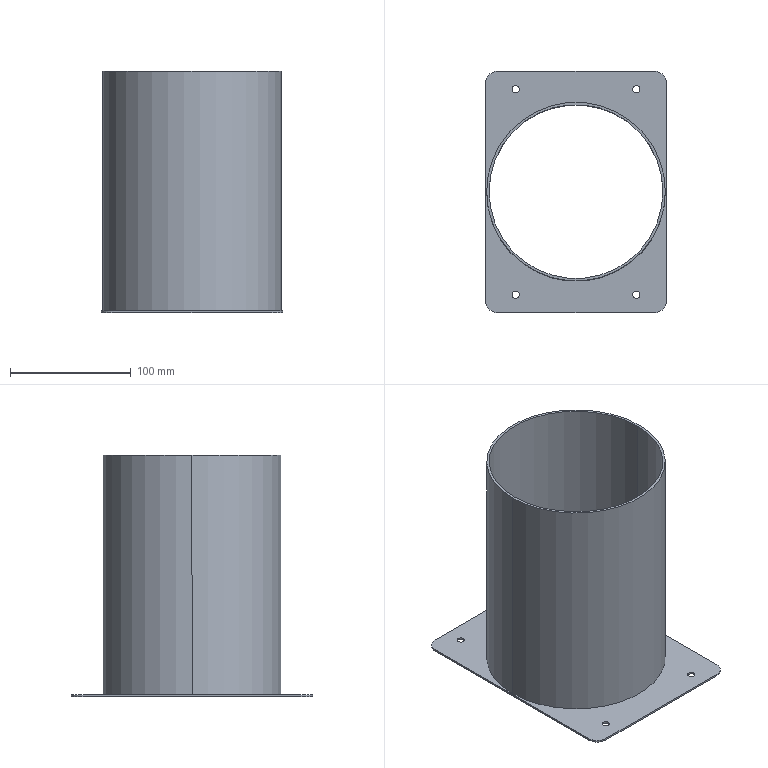Part | SolidWorks | features Extrusion 1, Fillet 1, HoleWzd 1, ICE 1 | 1 solid | 23 faces | box 150 x 200 x 200 mm | volume 202366 mm3 | cylinder 16 | plane 7 | commonest cylinder face diameters 6 x8 20 x4 144 x2 148 x2
STEP:
#1=CARTESIAN_POINT('',(-53.,-85.,0.));
#2=VERTEX_POINT('',#1);
#3=CARTESIAN_POINT('',(-47.,-85.,0.));
#4=VERTEX_POINT('',#3);
#5=CARTESIAN_POINT('',(-50.,-85.,0.));
#6=DIRECTION('',(0.,0.,1.));
#7=DIRECTION('',(1.,0.,0.));
#8=AXIS2_PLACEMENT_3D('',#5,#6,#7);
#9=CIRCLE('',#8,3.);
#10=EDGE_CURVE('',#2,#4,#9,.T.);
#11=ORIENTED_EDGE('',*,*,#10,.F.);
#12=CARTESIAN_POINT('',(-53.,-85.,1.5));
#13=VERTEX_POINT('',#12);
#14=CARTESIAN_POINT('',(-53.,-85.,1.5));
#15=DIRECTION('',(0.,0.,1.));
#16=VECTOR('',#15,1000.);
#17=LINE('',#14,#16);
#18=EDGE_CURVE('',#2,#13,#17,.T.);
#19=ORIENTED_EDGE('',*,*,#18,.T.);
#20=CARTESIAN_POINT('',(-47.,-85.,1.5));
#21=VERTEX_POINT('',#20);
#22=CARTESIAN_POINT('',(-50.,-85.,1.5));
#23=DIRECTION('',(0.,0.,1.));
#24=DIRECTION('',(1.,0.,0.));
#25=AXIS2_PLACEMENT_3D('',#22,#23,#24);
#26=CIRCLE('',#25,3.);
#27=EDGE_CURVE('',#13,#21,#26,.T.);
#28=ORIENTED_EDGE('',*,*,#27,.T.);
#29=CARTESIAN_POINT('',(-47.,-85.,1.5));
#30=DIRECTION('',(0.,0.,1.));
#31=VECTOR('',#30,1000.);
#32=LINE('',#29,#31);
#33=EDGE_CURVE('',#4,#21,#32,.T.);
#34=ORIENTED_EDGE('',*,*,#33,.F.);
#35=EDGE_LOOP('',(#11,#19,#28,#34));
#36=FACE_OUTER_BOUND('',#35,.T.);
#37=CARTESIAN_POINT('',(-50.,-85.,1.5));
#38=DIRECTION('',(0.,0.,1.));
#39=DIRECTION('',(1.,0.,0.));
#40=AXIS2_PLACEMENT_3D('',#37,#38,#39);
#41=CYLINDRICAL_SURFACE('',#40,3.);
#42=ADVANCED_FACE('',(#36),#41,.F.);
#43=CARTESIAN_POINT('',(-53.,85.,0.));
#44=VERTEX_POINT('',#43);
#45=CARTESIAN_POINT('',(-47.,85.,0.));
#46=VERTEX_POINT('',#45);
#47=CARTESIAN_POINT('',(-50.,85.,0.));
#48=DIRECTION('',(0.,0.,1.));
#49=DIRECTION('',(1.,0.,0.));
#50=AXIS2_PLACEMENT_3D('',#47,#48,#49);
#51=CIRCLE('',#50,3.);
#52=EDGE_CURVE('',#44,#46,#51,.T.);
#53=ORIENTED_EDGE('',*,*,#52,.F.);
#54=CARTESIAN_POINT('',(-53.,85.,1.5));
#55=VERTEX_POINT('',#54);
#56=CARTESIAN_POINT('',(-53.,85.,1.5));
#57=DIRECTION('',(0.,0.,1.));
#58=VECTOR('',#57,1000.);
#59=LINE('',#56,#58);
#60=EDGE_CURVE('',#44,#55,#59,.T.);
#61=ORIENTED_EDGE('',*,*,#60,.T.);
#62=CARTESIAN_POINT('',(-47.,85.,1.5));
#63=VERTEX_POINT('',#62);
#64=CARTESIAN_POINT('',(-50.,85.,1.5));
#65=DIRECTION('',(0.,0.,1.));
#66=DIRECTION('',(1.,0.,0.));
#67=AXIS2_PLACEMENT_3D('',#64,#65,#66);
#68=CIRCLE('',#67,3.);
#69=EDGE_CURVE('',#55,#63,#68,.T.);
#70=ORIENTED_EDGE('',*,*,#69,.T.);
#71=CARTESIAN_POINT('',(-47.,85.,1.5));
#72=DIRECTION('',(0.,0.,1.));
#73=VECTOR('',#72,1000.);
#74=LINE('',#71,#73);
#75=EDGE_CURVE('',#46,#63,#74,.T.);
#76=ORIENTED_EDGE('',*,*,#75,.F.);
#77=EDGE_LOOP('',(#53,#61,#70,#76));
#78=FACE_OUTER_BOUND('',#77,.T.);
#79=CARTESIAN_POINT('',(-50.,85.,1.5));
#80=DIRECTION('',(0.,0.,1.));
#81=DIRECTION('',(1.,0.,0.));
#82=AXIS2_PLACEMENT_3D('',#79,#80,#81);
#83=CYLINDRICAL_SURFACE('',#82,3.);
#84=ADVANCED_FACE('',(#78),#83,.F.);
#85=CARTESIAN_POINT('',(47.,85.,0.));
#86=VERTEX_POINT('',#85);
#87=CARTESIAN_POINT('',(53.,85.,0.));
#88=VERTEX_POINT('',#87);
#89=CARTESIAN_POINT('',(50.,85.,0.));
#90=DIRECTION('',(0.,0.,1.));
#91=DIRECTION('',(1.,0.,0.));
#92=AXIS2_PLACEMENT_3D('',#89,#90,#91);
#93=CIRCLE('',#92,3.);
#94=EDGE_CURVE('',#86,#88,#93,.T.);
#95=ORIENTED_EDGE('',*,*,#94,.F.);
#96=CARTESIAN_POINT('',(47.,85.,1.5));
#97=VERTEX_POINT('',#96);
#98=CARTESIAN_POINT('',(47.,85.,1.5));
#99=DIRECTION('',(0.,0.,1.));
#100=VECTOR('',#99,1000.);
#101=LINE('',#98,#100);
#102=EDGE_CURVE('',#86,#97,#101,.T.);
#103=ORIENTED_EDGE('',*,*,#102,.T.);
#104=CARTESIAN_POINT('',(53.,85.,1.5));
#105=VERTEX_POINT('',#104);
#106=CARTESIAN_POINT('',(50.,85.,1.5));
#107=DIRECTION('',(0.,0.,1.));
#108=DIRECTION('',(1.,0.,0.));
#109=AXIS2_PLACEMENT_3D('',#106,#107,#108);
#110=CIRCLE('',#109,3.);
#111=EDGE_CURVE('',#97,#105,#110,.T.);
#112=ORIENTED_EDGE('',*,*,#111,.T.);
#113=CARTESIAN_POINT('',(53.,85.,1.5));
#114=DIRECTION('',(0.,0.,1.));
#115=VECTOR('',#114,1000.);
#116=LINE('',#113,#115);
#117=EDGE_CURVE('',#88,#105,#116,.T.);
#118=ORIENTED_EDGE('',*,*,#117,.F.);
#119=EDGE_LOOP('',(#95,#103,#112,#118));
#120=FACE_OUTER_BOUND('',#119,.T.);
#121=CARTESIAN_POINT('',(50.,85.,1.5));
#122=DIRECTION('',(0.,0.,1.));
#123=DIRECTION('',(1.,0.,0.));
#124=AXIS2_PLACEMENT_3D('',#121,#122,#123);
#125=CYLINDRICAL_SURFACE('',#124,3.);
#126=ADVANCED_FACE('',(#120),#125,.F.);
#127=CARTESIAN_POINT('',(47.,-85.,0.));
#128=VERTEX_POINT('',#127);
#129=CARTESIAN_POINT('',(53.,-85.,0.));
#130=VERTEX_POINT('',#129);
#131=CARTESIAN_POINT('',(50.,-85.,0.));
#132=DIRECTION('',(0.,0.,1.));
#133=DIRECTION('',(1.,0.,0.));
#134=AXIS2_PLACEMENT_3D('',#131,#132,#133);
#135=CIRCLE('',#134,3.);
#136=EDGE_CURVE('',#128,#130,#135,.T.);
#137=ORIENTED_EDGE('',*,*,#136,.F.);
#138=CARTESIAN_POINT('',(47.,-85.,1.5));
#139=VERTEX_POINT('',#138);
#140=CARTESIAN_POINT('',(47.,-85.,1.5));
#141=DIRECTION('',(0.,0.,1.));
#142=VECTOR('',#141,1000.);
#143=LINE('',#140,#142);
#144=EDGE_CURVE('',#128,#139,#143,.T.);
#145=ORIENTED_EDGE('',*,*,#144,.T.);
#146=CARTESIAN_POINT('',(53.,-85.,1.5));
#147=VERTEX_POINT('',#146);
#148=CARTESIAN_POINT('',(50.,-85.,1.5));
#149=DIRECTION('',(0.,0.,1.));
#150=DIRECTION('',(1.,0.,0.));
#151=AXIS2_PLACEMENT_3D('',#148,#149,#150);
#152=CIRCLE('',#151,3.);
#153=EDGE_CURVE('',#139,#147,#152,.T.);
#154=ORIENTED_EDGE('',*,*,#153,.T.);
#155=CARTESIAN_POINT('',(53.,-85.,1.5));
#156=DIRECTION('',(0.,0.,1.));
#157=VECTOR('',#156,1000.);
#158=LINE('',#155,#157);
#159=EDGE_CURVE('',#130,#147,#158,.T.);
#160=ORIENTED_EDGE('',*,*,#159,.F.);
#161=EDGE_LOOP('',(#137,#145,#154,#160));
#162=FACE_OUTER_BOUND('',#161,.T.);
#163=CARTESIAN_POINT('',(50.,-85.,1.5));
#164=DIRECTION('',(0.,0.,1.));
#165=DIRECTION('',(1.,0.,0.));
#166=AXIS2_PLACEMENT_3D('',#163,#164,#165);
#167=CYLINDRICAL_SURFACE('',#166,3.);
#168=ADVANCED_FACE('',(#162),#167,.F.);
#169=CARTESIAN_POINT('',(-72.,0.,200.));
#170=VERTEX_POINT('',#169);
#171=CARTESIAN_POINT('',(72.,0.,200.));
#172=VERTEX_POINT('',#171);
#173=CARTESIAN_POINT('',(0.,0.,200.));
#174=DIRECTION('',(0.,0.,1.));
#175=DIRECTION('',(1.,0.,0.));
#176=AXIS2_PLACEMENT_3D('',#173,#174,#175);
#177=CIRCLE('',#176,72.);
#178=EDGE_CURVE('',#170,#172,#177,.T.);
#179=ORIENTED_EDGE('',*,*,#178,.T.);
#180=CARTESIAN_POINT('',(72.,0.,0.));
#181=VERTEX_POINT('',#180);
#182=CARTESIAN_POINT('',(72.,0.,200.));
#183=DIRECTION('',(0.,0.,-1.));
#184=VECTOR('',#183,1000.);
#185=LINE('',#182,#184);
#186=EDGE_CURVE('',#172,#181,#185,.T.);
#187=ORIENTED_EDGE('',*,*,#186,.T.);
#188=CARTESIAN_POINT('',(-72.,0.,0.));
#189=VERTEX_POINT('',#188);
#190=CARTESIAN_POINT('',(0.,0.,0.));
#191=DIRECTION('',(0.,0.,1.));
#192=DIRECTION('',(1.,0.,0.));
#193=AXIS2_PLACEMENT_3D('',#190,#191,#192);
#194=CIRCLE('',#193,72.);
#195=EDGE_CURVE('',#189,#181,#194,.T.);
#196=ORIENTED_EDGE('',*,*,#195,.F.);
#197=CARTESIAN_POINT('',(-72.,0.,200.));
#198=DIRECTION('',(0.,0.,-1.));
#199=VECTOR('',#198,1000.);
#200=LINE('',#197,#199);
#201=EDGE_CURVE('',#170,#189,#200,.T.);
#202=ORIENTED_EDGE('',*,*,#201,.F.);
#203=EDGE_LOOP('',(#179,#187,#196,#202));
#204=FACE_OUTER_BOUND('',#203,.T.);
#205=CARTESIAN_POINT('',(0.,0.,200.));
#206=DIRECTION('',(0.,0.,-1.));
#207=DIRECTION('',(-1.,0.,0.));
#208=AXIS2_PLACEMENT_3D('',#205,#206,#207);
#209=CYLINDRICAL_SURFACE('',#208,72.);
#210=ADVANCED_FACE('',(#204),#209,.F.);
#211=CARTESIAN_POINT('',(74.,0.,200.));
#212=VERTEX_POINT('',#211);
#213=CARTESIAN_POINT('',(-74.,0.,200.));
#214=VERTEX_POINT('',#213);
#215=CARTESIAN_POINT('',(0.,0.,200.));
#216=DIRECTION('',(0.,0.,1.));
#217=DIRECTION('',(1.,0.,0.));
#218=AXIS2_PLACEMENT_3D('',#215,#216,#217);
#219=CIRCLE('',#218,74.);
#220=EDGE_CURVE('',#212,#214,#219,.T.);
#221=ORIENTED_EDGE('',*,*,#220,.F.);
#222=CARTESIAN_POINT('',(74.,0.,1.5));
#223=VERTEX_POINT('',#222);
#224=CARTESIAN_POINT('',(74.,0.,200.));
#225=DIRECTION('',(0.,0.,-1.));
#226=VECTOR('',#225,1000.);
#227=LINE('',#224,#226);
#228=EDGE_CURVE('',#212,#223,#227,.T.);
#229=ORIENTED_EDGE('',*,*,#228,.T.);
#230=CARTESIAN_POINT('',(-74.,0.,1.5));
#231=VERTEX_POINT('',#230);
#232=CARTESIAN_POINT('',(0.,0.,1.5));
#233=DIRECTION('',(0.,0.,-1.));
#234=DIRECTION('',(-1.,0.,0.));
#235=AXIS2_PLACEMENT_3D('',#232,#233,#234);
#236=CIRCLE('',#235,74.);
#237=EDGE_CURVE('',#231,#223,#236,.T.);
#238=ORIENTED_EDGE('',*,*,#237,.F.);
#239=CARTESIAN_POINT('',(-74.,0.,200.));
#240=DIRECTION('',(0.,0.,-1.));
#241=VECTOR('',#240,1000.);
#242=LINE('',#239,#241);
#243=EDGE_CURVE('',#214,#231,#242,.T.);
#244=ORIENTED_EDGE('',*,*,#243,.F.);
#245=EDGE_LOOP('',(#221,#229,#238,#244));
#246=FACE_OUTER_BOUND('',#245,.T.);
#247=CARTESIAN_POINT('',(0.,0.,200.));
#248=DIRECTION('',(0.,0.,-1.));
#249=DIRECTION('',(-1.,0.,0.));
#250=AXIS2_PLACEMENT_3D('',#247,#248,#249);
#251=CYLINDRICAL_SURFACE('',#250,74.);
#252=ADVANCED_FACE('',(#246),#251,.T.);
#253=CARTESIAN_POINT('',(0.,0.,200.));
#254=DIRECTION('',(0.,0.,1.));
#255=DIRECTION('',(1.,0.,0.));
#256=AXIS2_PLACEMENT_3D('',#253,#254,#255);
#257=CIRCLE('',#256,74.);
#258=EDGE_CURVE('',#214,#212,#257,.T.);
#259=ORIENTED_EDGE('',*,*,#258,.T.);
#260=ORIENTED_EDGE('',*,*,#220,.T.);
#261=EDGE_LOOP('',(#259,#260));
#262=FACE_OUTER_BOUND('',#261,.T.);
#263=ORIENTED_EDGE('',*,*,#178,.F.);
#264=CARTESIAN_POINT('',(0.,0.,200.));
#265=DIRECTION('',(0.,0.,1.));
#266=DIRECTION('',(1.,0.,0.));
#267=AXIS2_PLACEMENT_3D('',#264,#265,#266);
#268=CIRCLE('',#267,72.);
#269=EDGE_CURVE('',#172,#170,#268,.T.);
#270=ORIENTED_EDGE('',*,*,#269,.F.);
#271=EDGE_LOOP('',(#263,#270));
#272=FACE_BOUND('',#271,.T.);
#273=CARTESIAN_POINT('',(0.,0.,200.));
#274=DIRECTION('',(0.,0.,1.));
#275=DIRECTION('',(1.,0.,0.));
#276=AXIS2_PLACEMENT_3D('',#273,#274,#275);
#277=PLANE('',#276);
#278=ADVANCED_FACE('',(#262,#272),#277,.T.);
#279=CARTESIAN_POINT('',(-50.,-85.,0.));
#280=DIRECTION('',(0.,0.,1.));
#281=DIRECTION('',(1.,0.,0.));
#282=AXIS2_PLACEMENT_3D('',#279,#280,#281);
#283=CIRCLE('',#282,3.);
#284=EDGE_CURVE('',#4,#2,#283,.T.);
#285=ORIENTED_EDGE('',*,*,#284,.T.);
#286=ORIENTED_EDGE('',*,*,#10,.T.);
#287=EDGE_LOOP('',(#285,#286));
#288=FACE_BOUND('',#287,.T.);
#289=CARTESIAN_POINT('',(-50.,85.,0.));
#290=DIRECTION('',(0.,0.,1.));
#291=DIRECTION('',(1.,0.,0.));
#292=AXIS2_PLACEMENT_3D('',#289,#290,#291);
#293=CIRCLE('',#292,3.);
#294=EDGE_CURVE('',#46,#44,#293,.T.);
#295=ORIENTED_EDGE('',*,*,#294,.T.);
#296=ORIENTED_EDGE('',*,*,#52,.T.);
#297=EDGE_LOOP('',(#295,#296));
#298=FACE_BOUND('',#297,.T.);
#299=CARTESIAN_POINT('',(50.,85.,0.));
#300=DIRECTION('',(0.,0.,1.));
#301=DIRECTION('',(1.,0.,0.));
#302=AXIS2_PLACEMENT_3D('',#299,#300,#301);
#303=CIRCLE('',#302,3.);
#304=EDGE_CURVE('',#88,#86,#303,.T.);
#305=ORIENTED_EDGE('',*,*,#304,.T.);
#306=ORIENTED_EDGE('',*,*,#94,.T.);
#307=EDGE_LOOP('',(#305,#306));
#308=FACE_BOUND('',#307,.T.);
#309=CARTESIAN_POINT('',(50.,-85.,0.));
#310=DIRECTION('',(0.,0.,1.));
#311=DIRECTION('',(1.,0.,0.));
#312=AXIS2_PLACEMENT_3D('',#309,#310,#311);
#313=CIRCLE('',#312,3.);
#314=EDGE_CURVE('',#130,#128,#313,.T.);
#315=ORIENTED_EDGE('',*,*,#314,.T.);
#316=ORIENTED_EDGE('',*,*,#136,.T.);
#317=EDGE_LOOP('',(#315,#316));
#318=FACE_BOUND('',#317,.T.);
#319=ORIENTED_EDGE('',*,*,#195,.T.);
#320=CARTESIAN_POINT('',(0.,0.,0.));
#321=DIRECTION('',(0.,0.,1.));
#322=DIRECTION('',(1.,0.,0.));
#323=AXIS2_PLACEMENT_3D('',#320,#321,#322);
#324=CIRCLE('',#323,72.);
#325=EDGE_CURVE('',#181,#189,#324,.T.);
#326=ORIENTED_EDGE('',*,*,#325,.T.);
#327=EDGE_LOOP('',(#319,#326));
#328=FACE_BOUND('',#327,.T.);
#329=CARTESIAN_POINT('',(-65.,100.,0.));
#330=VERTEX_POINT('',#329);
#331=CARTESIAN_POINT('',(65.,100.,0.));
#332=VERTEX_POINT('',#331);
#333=CARTESIAN_POINT('',(75.,100.,0.));
#334=DIRECTION('',(1.,0.,0.));
#335=VECTOR('',#334,1000.);
#336=LINE('',#333,#335);
#337=EDGE_CURVE('',#330,#332,#336,.T.);
#338=ORIENTED_EDGE('',*,*,#337,.T.);
#339=CARTESIAN_POINT('',(75.,90.,0.));
#340=VERTEX_POINT('',#339);
#341=CARTESIAN_POINT('',(65.,90.,0.));
#342=DIRECTION('',(0.,0.,-1.));
#343=DIRECTION('',(1.,0.,0.));
#344=AXIS2_PLACEMENT_3D('',#341,#342,#343);
#345=CIRCLE('',#344,10.);
#346=EDGE_CURVE('',#332,#340,#345,.T.);
#347=ORIENTED_EDGE('',*,*,#346,.T.);
#348=CARTESIAN_POINT('',(75.,-90.,0.));
#349=VERTEX_POINT('',#348);
#350=CARTESIAN_POINT('',(75.,-100.,0.));
#351=DIRECTION('',(0.,-1.,0.));
#352=VECTOR('',#351,1000.);
#353=LINE('',#350,#352);
#354=EDGE_CURVE('',#340,#349,#353,.T.);
#355=ORIENTED_EDGE('',*,*,#354,.T.);
#356=CARTESIAN_POINT('',(65.,-100.,0.));
#357=VERTEX_POINT('',#356);
#358=CARTESIAN_POINT('',(65.,-90.,0.));
#359=DIRECTION('',(0.,0.,-1.));
#360=DIRECTION('',(1.,0.,0.));
#361=AXIS2_PLACEMENT_3D('',#358,#359,#360);
#362=CIRCLE('',#361,10.);
#363=EDGE_CURVE('',#349,#357,#362,.T.);
#364=ORIENTED_EDGE('',*,*,#363,.T.);
#365=CARTESIAN_POINT('',(-65.,-100.,0.));
#366=VERTEX_POINT('',#365);
#367=CARTESIAN_POINT('',(75.,-100.,0.));
#368=DIRECTION('',(-1.,0.,0.));
#369=VECTOR('',#368,1000.);
#370=LINE('',#367,#369);
#371=EDGE_CURVE('',#357,#366,#370,.T.);
#372=ORIENTED_EDGE('',*,*,#371,.T.);
#373=CARTESIAN_POINT('',(-75.,-90.,0.));
#374=VERTEX_POINT('',#373);
#375=CARTESIAN_POINT('',(-65.,-90.,0.));
#376=DIRECTION('',(0.,0.,-1.));
#377=DIRECTION('',(1.,0.,0.));
#378=AXIS2_PLACEMENT_3D('',#375,#376,#377);
#379=CIRCLE('',#378,10.);
#380=EDGE_CURVE('',#366,#374,#379,.T.);
#381=ORIENTED_EDGE('',*,*,#380,.T.);
#382=CARTESIAN_POINT('',(-75.,90.,0.));
#383=VERTEX_POINT('',#382);
#384=CARTESIAN_POINT('',(-75.,-100.,0.));
#385=DIRECTION('',(0.,1.,0.));
#386=VECTOR('',#385,1000.);
#387=LINE('',#384,#386);
#388=EDGE_CURVE('',#374,#383,#387,.T.);
#389=ORIENTED_EDGE('',*,*,#388,.T.);
#390=CARTESIAN_POINT('',(-65.,90.,0.));
#391=DIRECTION('',(0.,0.,-1.));
#392=DIRECTION('',(1.,0.,0.));
#393=AXIS2_PLACEMENT_3D('',#390,#391,#392);
#394=CIRCLE('',#393,10.);
#395=EDGE_CURVE('',#383,#330,#394,.T.);
#396=ORIENTED_EDGE('',*,*,#395,.T.);
#397=EDGE_LOOP('',(#338,#347,#355,#364,#372,#381,#389,#396));
#398=FACE_OUTER_BOUND('',#397,.T.);
#399=CARTESIAN_POINT('',(0.,0.,0.));
#400=DIRECTION('',(0.,0.,1.));
#401=DIRECTION('',(1.,0.,0.));
#402=AXIS2_PLACEMENT_3D('',#399,#400,#401);
#403=PLANE('',#402);
#404=ADVANCED_FACE('',(#288,#298,#308,#318,#328,#398),#403,.F.);
#405=ORIENTED_EDGE('',*,*,#228,.F.);
#406=ORIENTED_EDGE('',*,*,#258,.F.);
#407=ORIENTED_EDGE('',*,*,#243,.T.);
#408=CARTESIAN_POINT('',(0.,0.,1.5));
#409=DIRECTION('',(0.,0.,-1.));
#410=DIRECTION('',(-1.,0.,0.));
#411=AXIS2_PLACEMENT_3D('',#408,#409,#410);
#412=CIRCLE('',#411,74.);
#413=EDGE_CURVE('',#223,#231,#412,.T.);
#414=ORIENTED_EDGE('',*,*,#413,.F.);
#415=EDGE_LOOP('',(#405,#406,#407,#414));
#416=FACE_OUTER_BOUND('',#415,.T.);
#417=CARTESIAN_POINT('',(0.,0.,200.));
#418=DIRECTION('',(0.,0.,-1.));
#419=DIRECTION('',(-1.,0.,0.));
#420=AXIS2_PLACEMENT_3D('',#417,#418,#419);
#421=CYLINDRICAL_SURFACE('',#420,74.);
#422=ADVANCED_FACE('',(#416),#421,.T.);
#423=ORIENTED_EDGE('',*,*,#186,.F.);
#424=ORIENTED_EDGE('',*,*,#269,.T.);
#425=ORIENTED_EDGE('',*,*,#201,.T.);
#426=ORIENTED_EDGE('',*,*,#325,.F.);
#427=EDGE_LOOP('',(#423,#424,#425,#426));
#428=FACE_OUTER_BOUND('',#427,.T.);
#429=CARTESIAN_POINT('',(0.,0.,200.));
#430=DIRECTION('',(0.,0.,-1.));
#431=DIRECTION('',(-1.,0.,0.));
#432=AXIS2_PLACEMENT_3D('',#429,#430,#431);
#433=CYLINDRICAL_SURFACE('',#432,72.);
#434=ADVANCED_FACE('',(#428),#433,.F.);
#435=ORIENTED_EDGE('',*,*,#388,.F.);
#436=CARTESIAN_POINT('',(-75.,-90.,1.5));
#437=VERTEX_POINT('',#436);
#438=CARTESIAN_POINT('',(-75.,-90.,1.5));
#439=DIRECTION('',(0.,0.,1.));
#440=VECTOR('',#439,1000.);
#441=LINE('',#438,#440);
#442=EDGE_CURVE('',#374,#437,#441,.T.);
#443=ORIENTED_EDGE('',*,*,#442,.T.);
#444=CARTESIAN_POINT('',(-75.,90.,1.5));
#445=VERTEX_POINT('',#444);
#446=CARTESIAN_POINT('',(-75.,-100.,1.5));
#447=DIRECTION('',(0.,1.,0.));
#448=VECTOR('',#447,1000.);
#449=LINE('',#446,#448);
#450=EDGE_CURVE('',#437,#445,#449,.T.);
#451=ORIENTED_EDGE('',*,*,#450,.T.);
#452=CARTESIAN_POINT('',(-75.,90.,1.5));
#453=DIRECTION('',(0.,0.,-1.));
#454=VECTOR('',#453,1000.);
#455=LINE('',#452,#454);
#456=EDGE_CURVE('',#445,#383,#455,.T.);
#457=ORIENTED_EDGE('',*,*,#456,.T.);
#458=EDGE_LOOP('',(#435,#443,#451,#457));
#459=FACE_OUTER_BOUND('',#458,.T.);
#460=CARTESIAN_POINT('',(-75.,-100.,1.5));
#461=DIRECTION('',(-1.,0.,0.));
#462=DIRECTION('',(0.,0.,1.));
#463=AXIS2_PLACEMENT_3D('',#460,#461,#462);
#464=PLANE('',#463);
#465=ADVANCED_FACE('',(#459),#464,.T.);
#466=ORIENTED_EDGE('',*,*,#371,.F.);
#467=CARTESIAN_POINT('',(65.,-100.,1.5));
#468=VERTEX_POINT('',#467);
#469=CARTESIAN_POINT('',(65.,-100.,1.5));
#470=DIRECTION('',(0.,0.,1.));
#471=VECTOR('',#470,1000.);
#472=LINE('',#469,#471);
#473=EDGE_CURVE('',#357,#468,#472,.T.);
#474=ORIENTED_EDGE('',*,*,#473,.T.);
#475=CARTESIAN_POINT('',(-65.,-100.,1.5));
#476=VERTEX_POINT('',#475);
#477=CARTESIAN_POINT('',(75.,-100.,1.5));
#478=DIRECTION('',(-1.,0.,0.));
#479=VECTOR('',#478,1000.);
#480=LINE('',#477,#479);
#481=EDGE_CURVE('',#468,#476,#480,.T.);
#482=ORIENTED_EDGE('',*,*,#481,.T.);
#483=CARTESIAN_POINT('',(-65.,-100.,1.5));
#484=DIRECTION('',(0.,0.,-1.));
#485=VECTOR('',#484,1000.);
#486=LINE('',#483,#485);
#487=EDGE_CURVE('',#476,#366,#486,.T.);
#488=ORIENTED_EDGE('',*,*,#487,.T.);
#489=EDGE_LOOP('',(#466,#474,#482,#488));
#490=FACE_OUTER_BOUND('',#489,.T.);
#491=CARTESIAN_POINT('',(75.,-100.,1.5));
#492=DIRECTION('',(0.,-1.,0.));
#493=DIRECTION('',(0.,0.,-1.));
#494=AXIS2_PLACEMENT_3D('',#491,#492,#493);
#495=PLANE('',#494);
#496=ADVANCED_FACE('',(#490),#495,.T.);
#497=ORIENTED_EDGE('',*,*,#354,.F.);
#498=CARTESIAN_POINT('',(75.,90.,1.5));
#499=VERTEX_POINT('',#498);
#500=CARTESIAN_POINT('',(75.,90.,1.5));
#501=DIRECTION('',(0.,0.,1.));
#502=VECTOR('',#501,1000.);
#503=LINE('',#500,#502);
#504=EDGE_CURVE('',#340,#499,#503,.T.);
#505=ORIENTED_EDGE('',*,*,#504,.T.);
#506=CARTESIAN_POINT('',(75.,-90.,1.5));
#507=VERTEX_POINT('',#506);
#508=CARTESIAN_POINT('',(75.,-100.,1.5));
#509=DIRECTION('',(0.,-1.,0.));
#510=VECTOR('',#509,1000.);
#511=LINE('',#508,#510);
#512=EDGE_CURVE('',#499,#507,#511,.T.);
#513=ORIENTED_EDGE('',*,*,#512,.T.);
#514=CARTESIAN_POINT('',(75.,-90.,1.5));
#515=DIRECTION('',(0.,0.,-1.));
#516=VECTOR('',#515,1000.);
#517=LINE('',#514,#516);
#518=EDGE_CURVE('',#507,#349,#517,.T.);
#519=ORIENTED_EDGE('',*,*,#518,.T.);
#520=EDGE_LOOP('',(#497,#505,#513,#519));
#521=FACE_OUTER_BOUND('',#520,.T.);
#522=CARTESIAN_POINT('',(75.,-100.,1.5));
#523=DIRECTION('',(1.,0.,0.));
#524=DIRECTION('',(0.,0.,-1.));
#525=AXIS2_PLACEMENT_3D('',#522,#523,#524);
#526=PLANE('',#525);
#527=ADVANCED_FACE('',(#521),#526,.T.);
#528=CARTESIAN_POINT('',(-65.,100.,1.5));
#529=VERTEX_POINT('',#528);
#530=CARTESIAN_POINT('',(65.,100.,1.5));
#531=VERTEX_POINT('',#530);
#532=CARTESIAN_POINT('',(75.,100.,1.5));
#533=DIRECTION('',(1.,0.,0.));
#534=VECTOR('',#533,1000.);
#535=LINE('',#532,#534);
#536=EDGE_CURVE('',#529,#531,#535,.T.);
#537=ORIENTED_EDGE('',*,*,#536,.T.);
#538=CARTESIAN_POINT('',(65.,100.,1.5));
#539=DIRECTION('',(0.,0.,-1.));
#540=VECTOR('',#539,1000.);
#541=LINE('',#538,#540);
#542=EDGE_CURVE('',#531,#332,#541,.T.);
#543=ORIENTED_EDGE('',*,*,#542,.T.);
#544=ORIENTED_EDGE('',*,*,#337,.F.);
#545=CARTESIAN_POINT('',(-65.,100.,1.5));
#546=DIRECTION('',(0.,0.,1.));
#547=VECTOR('',#546,1000.);
#548=LINE('',#545,#547);
#549=EDGE_CURVE('',#330,#529,#548,.T.);
#550=ORIENTED_EDGE('',*,*,#549,.T.);
#551=EDGE_LOOP('',(#537,#543,#544,#550));
#552=FACE_OUTER_BOUND('',#551,.T.);
#553=CARTESIAN_POINT('',(75.,100.,1.5));
#554=DIRECTION('',(0.,1.,0.));
#555=DIRECTION('',(0.,0.,1.));
#556=AXIS2_PLACEMENT_3D('',#553,#554,#555);
#557=PLANE('',#556);
#558=ADVANCED_FACE('',(#552),#557,.T.);
#559=CARTESIAN_POINT('',(-50.,-85.,1.5));
#560=DIRECTION('',(0.,0.,1.));
#561=DIRECTION('',(1.,0.,0.));
#562=AXIS2_PLACEMENT_3D('',#559,#560,#561);
#563=CIRCLE('',#562,3.);
#564=EDGE_CURVE('',#21,#13,#563,.T.);
#565=ORIENTED_EDGE('',*,*,#564,.F.);
#566=ORIENTED_EDGE('',*,*,#27,.F.);
#567=EDGE_LOOP('',(#565,#566));
#568=FACE_BOUND('',#567,.T.);
#569=CARTESIAN_POINT('',(-50.,85.,1.5));
#570=DIRECTION('',(0.,0.,1.));
#571=DIRECTION('',(1.,0.,0.));
#572=AXIS2_PLACEMENT_3D('',#569,#570,#571);
#573=CIRCLE('',#572,3.);
#574=EDGE_CURVE('',#63,#55,#573,.T.);
#575=ORIENTED_EDGE('',*,*,#574,.F.);
#576=ORIENTED_EDGE('',*,*,#69,.F.);
#577=EDGE_LOOP('',(#575,#576));
#578=FACE_BOUND('',#577,.T.);
#579=CARTESIAN_POINT('',(50.,85.,1.5));
#580=DIRECTION('',(0.,0.,1.));
#581=DIRECTION('',(1.,0.,0.));
#582=AXIS2_PLACEMENT_3D('',#579,#580,#581);
#583=CIRCLE('',#582,3.);
#584=EDGE_CURVE('',#105,#97,#583,.T.);
#585=ORIENTED_EDGE('',*,*,#584,.F.);
#586=ORIENTED_EDGE('',*,*,#111,.F.);
#587=EDGE_LOOP('',(#585,#586));
#588=FACE_BOUND('',#587,.T.);
#589=CARTESIAN_POINT('',(50.,-85.,1.5));
#590=DIRECTION('',(0.,0.,1.));
#591=DIRECTION('',(1.,0.,0.));
#592=AXIS2_PLACEMENT_3D('',#589,#590,#591);
#593=CIRCLE('',#592,3.);
#594=EDGE_CURVE('',#147,#139,#593,.T.);
#595=ORIENTED_EDGE('',*,*,#594,.F.);
#596=ORIENTED_EDGE('',*,*,#153,.F.);
#597=EDGE_LOOP('',(#595,#596));
#598=FACE_BOUND('',#597,.T.);
#599=ORIENTED_EDGE('',*,*,#237,.T.);
#600=ORIENTED_EDGE('',*,*,#413,.T.);
#601=EDGE_LOOP('',(#599,#600));
#602=FACE_BOUND('',#601,.T.);
#603=ORIENTED_EDGE('',*,*,#512,.F.);
#604=CARTESIAN_POINT('',(65.,90.,1.5));
#605=DIRECTION('',(0.,0.,1.));
#606=DIRECTION('',(1.,0.,0.));
#607=AXIS2_PLACEMENT_3D('',#604,#605,#606);
#608=CIRCLE('',#607,10.);
#609=EDGE_CURVE('',#499,#531,#608,.T.);
#610=ORIENTED_EDGE('',*,*,#609,.T.);
#611=ORIENTED_EDGE('',*,*,#536,.F.);
#612=CARTESIAN_POINT('',(-65.,90.,1.5));
#613=DIRECTION('',(0.,0.,1.));
#614=DIRECTION('',(1.,0.,0.));
#615=AXIS2_PLACEMENT_3D('',#612,#613,#614);
#616=CIRCLE('',#615,10.);
#617=EDGE_CURVE('',#529,#445,#616,.T.);
#618=ORIENTED_EDGE('',*,*,#617,.T.);
#619=ORIENTED_EDGE('',*,*,#450,.F.);
#620=CARTESIAN_POINT('',(-65.,-90.,1.5));
#621=DIRECTION('',(0.,0.,1.));
#622=DIRECTION('',(1.,0.,0.));
#623=AXIS2_PLACEMENT_3D('',#620,#621,#622);
#624=CIRCLE('',#623,10.);
#625=EDGE_CURVE('',#437,#476,#624,.T.);
#626=ORIENTED_EDGE('',*,*,#625,.T.);
#627=ORIENTED_EDGE('',*,*,#481,.F.);
#628=CARTESIAN_POINT('',(65.,-90.,1.5));
#629=DIRECTION('',(0.,0.,1.));
#630=DIRECTION('',(1.,0.,0.));
#631=AXIS2_PLACEMENT_3D('',#628,#629,#630);
#632=CIRCLE('',#631,10.);
#633=EDGE_CURVE('',#468,#507,#632,.T.);
#634=ORIENTED_EDGE('',*,*,#633,.T.);
#635=EDGE_LOOP('',(#603,#610,#611,#618,#619,#626,#627,#634));
#636=FACE_OUTER_BOUND('',#635,.T.);
#637=CARTESIAN_POINT('',(0.,0.,1.5));
#638=DIRECTION('',(0.,0.,1.));
#639=DIRECTION('',(1.,0.,0.));
#640=AXIS2_PLACEMENT_3D('',#637,#638,#639);
#641=PLANE('',#640);
#642=ADVANCED_FACE('',(#568,#578,#588,#598,#602,#636),#641,.T.);
#643=ORIENTED_EDGE('',*,*,#609,.F.);
#644=ORIENTED_EDGE('',*,*,#504,.F.);
#645=ORIENTED_EDGE('',*,*,#346,.F.);
#646=ORIENTED_EDGE('',*,*,#542,.F.);
#647=EDGE_LOOP('',(#643,#644,#645,#646));
#648=FACE_OUTER_BOUND('',#647,.T.);
#649=CARTESIAN_POINT('',(65.,90.,1.5));
#650=DIRECTION('',(0.,0.,-1.));
#651=DIRECTION('',(-1.,0.,0.));
#652=AXIS2_PLACEMENT_3D('',#649,#650,#651);
#653=CYLINDRICAL_SURFACE('',#652,10.);
#654=ADVANCED_FACE('',(#648),#653,.T.);
#655=ORIENTED_EDGE('',*,*,#633,.F.);
#656=ORIENTED_EDGE('',*,*,#473,.F.);
#657=ORIENTED_EDGE('',*,*,#363,.F.);
#658=ORIENTED_EDGE('',*,*,#518,.F.);
#659=EDGE_LOOP('',(#655,#656,#657,#658));
#660=FACE_OUTER_BOUND('',#659,.T.);
#661=CARTESIAN_POINT('',(65.,-90.,1.5));
#662=DIRECTION('',(0.,0.,-1.));
#663=DIRECTION('',(-1.,0.,0.));
#664=AXIS2_PLACEMENT_3D('',#661,#662,#663);
#665=CYLINDRICAL_SURFACE('',#664,10.);
#666=ADVANCED_FACE('',(#660),#665,.T.);
#667=ORIENTED_EDGE('',*,*,#625,.F.);
#668=ORIENTED_EDGE('',*,*,#442,.F.);
#669=ORIENTED_EDGE('',*,*,#380,.F.);
#670=ORIENTED_EDGE('',*,*,#487,.F.);
#671=EDGE_LOOP('',(#667,#668,#669,#670));
#672=FACE_OUTER_BOUND('',#671,.T.);
#673=CARTESIAN_POINT('',(-65.,-90.,1.5));
#674=DIRECTION('',(0.,0.,-1.));
#675=DIRECTION('',(-1.,0.,0.));
#676=AXIS2_PLACEMENT_3D('',#673,#674,#675);
#677=CYLINDRICAL_SURFACE('',#676,10.);
#678=ADVANCED_FACE('',(#672),#677,.T.);
#679=ORIENTED_EDGE('',*,*,#617,.F.);
#680=ORIENTED_EDGE('',*,*,#549,.F.);
#681=ORIENTED_EDGE('',*,*,#395,.F.);
#682=ORIENTED_EDGE('',*,*,#456,.F.);
#683=EDGE_LOOP('',(#679,#680,#681,#682));
#684=FACE_OUTER_BOUND('',#683,.T.);
#685=CARTESIAN_POINT('',(-65.,90.,1.5));
#686=DIRECTION('',(0.,0.,-1.));
#687=DIRECTION('',(-1.,0.,0.));
#688=AXIS2_PLACEMENT_3D('',#685,#686,#687);
#689=CYLINDRICAL_SURFACE('',#688,10.);
#690=ADVANCED_FACE('',(#684),#689,.T.);
#691=ORIENTED_EDGE('',*,*,#144,.F.);
#692=ORIENTED_EDGE('',*,*,#314,.F.);
#693=ORIENTED_EDGE('',*,*,#159,.T.);
#694=ORIENTED_EDGE('',*,*,#594,.T.);
#695=EDGE_LOOP('',(#691,#692,#693,#694));
#696=FACE_OUTER_BOUND('',#695,.T.);
#697=CARTESIAN_POINT('',(50.,-85.,1.5));
#698=DIRECTION('',(0.,0.,1.));
#699=DIRECTION('',(1.,0.,0.));
#700=AXIS2_PLACEMENT_3D('',#697,#698,#699);
#701=CYLINDRICAL_SURFACE('',#700,3.);
#702=ADVANCED_FACE('',(#696),#701,.F.);
#703=ORIENTED_EDGE('',*,*,#102,.F.);
#704=ORIENTED_EDGE('',*,*,#304,.F.);
#705=ORIENTED_EDGE('',*,*,#117,.T.);
#706=ORIENTED_EDGE('',*,*,#584,.T.);
#707=EDGE_LOOP('',(#703,#704,#705,#706));
#708=FACE_OUTER_BOUND('',#707,.T.);
#709=CARTESIAN_POINT('',(50.,85.,1.5));
#710=DIRECTION('',(0.,0.,1.));
#711=DIRECTION('',(1.,0.,0.));
#712=AXIS2_PLACEMENT_3D('',#709,#710,#711);
#713=CYLINDRICAL_SURFACE('',#712,3.);
#714=ADVANCED_FACE('',(#708),#713,.F.);
#715=ORIENTED_EDGE('',*,*,#60,.F.);
#716=ORIENTED_EDGE('',*,*,#294,.F.);
#717=ORIENTED_EDGE('',*,*,#75,.T.);
#718=ORIENTED_EDGE('',*,*,#574,.T.);
#719=EDGE_LOOP('',(#715,#716,#717,#718));
#720=FACE_OUTER_BOUND('',#719,.T.);
#721=CARTESIAN_POINT('',(-50.,85.,1.5));
#722=DIRECTION('',(0.,0.,1.));
#723=DIRECTION('',(1.,0.,0.));
#724=AXIS2_PLACEMENT_3D('',#721,#722,#723);
#725=CYLINDRICAL_SURFACE('',#724,3.);
#726=ADVANCED_FACE('',(#720),#725,.F.);
#727=ORIENTED_EDGE('',*,*,#18,.F.);
#728=ORIENTED_EDGE('',*,*,#284,.F.);
#729=ORIENTED_EDGE('',*,*,#33,.T.);
#730=ORIENTED_EDGE('',*,*,#564,.T.);
#731=EDGE_LOOP('',(#727,#728,#729,#730));
#732=FACE_OUTER_BOUND('',#731,.T.);
#733=CARTESIAN_POINT('',(-50.,-85.,1.5));
#734=DIRECTION('',(0.,0.,1.));
#735=DIRECTION('',(1.,0.,0.));
#736=AXIS2_PLACEMENT_3D('',#733,#734,#735);
#737=CYLINDRICAL_SURFACE('',#736,3.);
#738=ADVANCED_FACE('',(#732),#737,.F.);
#739=CLOSED_SHELL('',(#42,#84,#126,#168,#210,#252,#278,#404,#422,#434,#465,#496,#527,#558,#642,#654,#666,#678,#690,#702,#714,#726,#738));
#740=MANIFOLD_SOLID_BREP('',#739);
#741=CARTESIAN_POINT('',(0.,0.,0.));
#742=DIRECTION('',(0.,0.,1.));
#743=DIRECTION('',(1.,0.,0.));
#744=AXIS2_PLACEMENT_3D('',#741,#742,#743);
#745=(LENGTH_UNIT()NAMED_UNIT(*)SI_UNIT(.MILLI.,.METRE.));
#746=UNCERTAINTY_MEASURE_WITH_UNIT(LENGTH_MEASURE(0.00001),#745,'','');
#747=(NAMED_UNIT(*)PLANE_ANGLE_UNIT()SI_UNIT($,.RADIAN.));
#748=(NAMED_UNIT(*)SI_UNIT($,.STERADIAN.)SOLID_ANGLE_UNIT());
#749=(GEOMETRIC_REPRESENTATION_CONTEXT(3)GLOBAL_UNCERTAINTY_ASSIGNED_CONTEXT((#746))GLOBAL_UNIT_ASSIGNED_CONTEXT((#745,#747,#748))REPRESENTATION_CONTEXT('',''));
#750=ADVANCED_BREP_SHAPE_REPRESENTATION('',(#740,#744),#749);